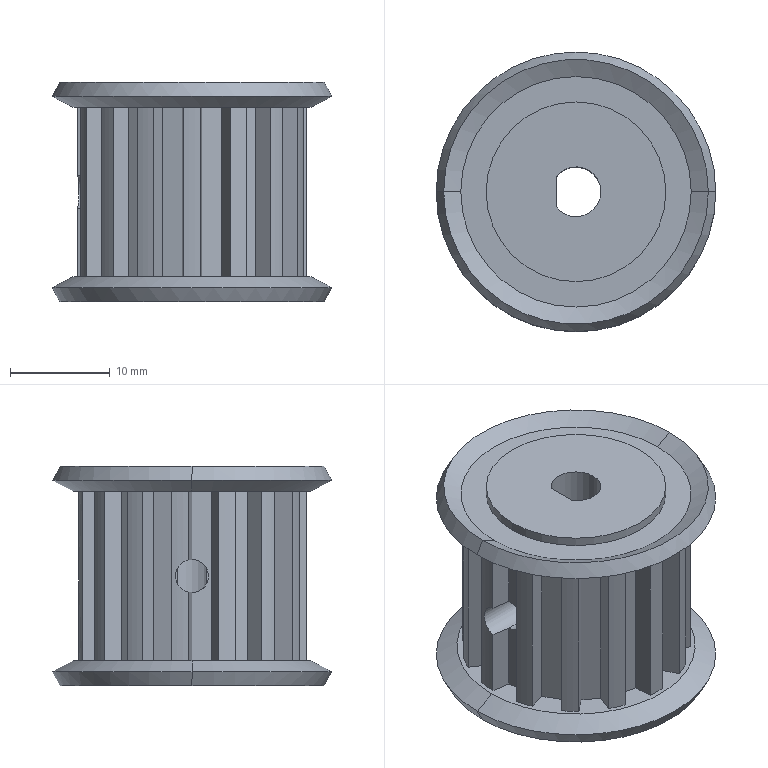Part | NX | features BREP 1 | 1 solid | 97 faces | box 28 x 28 x 22 mm | volume 7585 mm3 | plane 61 | cylinder 24 | cone 12 | commonest cylinder face diameters 22.91 x15 3.3 x4 18 x4 5 x1